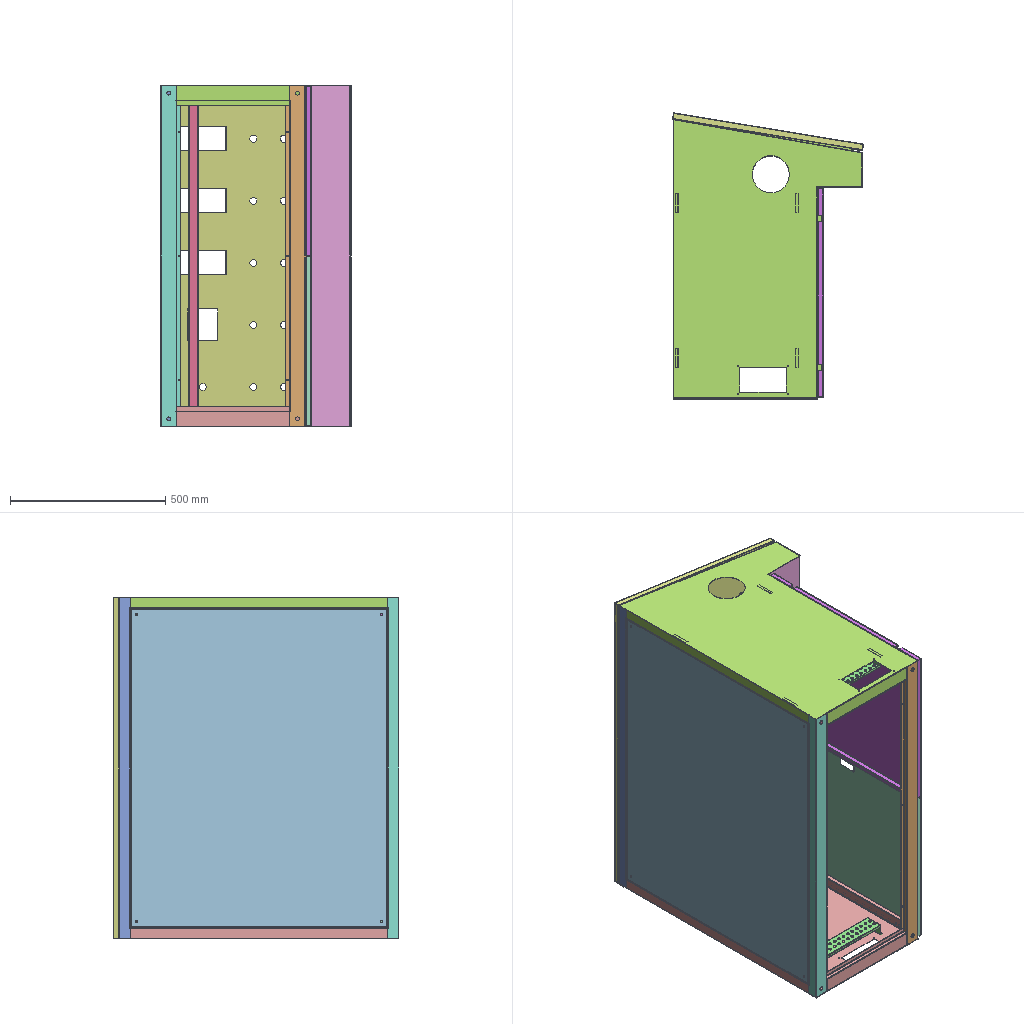Assembly | SolidWorks | 19 different items | 25 placed | box 615 x 920 x 1100 mm
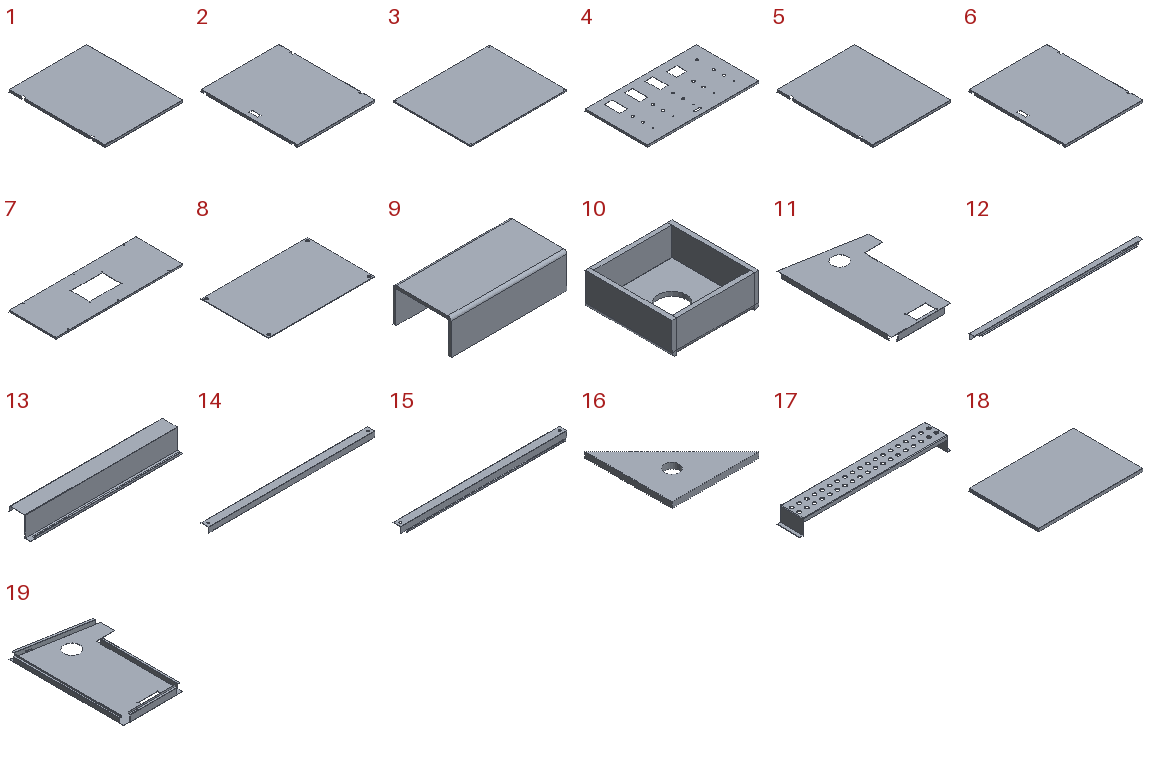Parts list (item | name | quantity | parent item | size | volume | features):
1 | (subassembly) | x1 | - | 559 x 672 x 18.5 mm | 634923 mm3 | -
2 | (subassembly) | x1 | - | 545.5 x 674 x 16.5 mm | 628405 mm3 | -
3 | - | x1 | - | 1027 x 827 x 13 mm | 1380132 mm3 | features EdgeFlange 2, FlatPattern 1, ICE 1, SMBaseFlange 1, SheetMetal 1
4 | - | x1 | - | 1100 x 620 x 20 mm | 1080338 mm3 | features EdgeFlange 2, ICE 2, FlatPattern 1, SMBaseFlange 1, SheetMetal 1
5 | - | x1 | in 1 | 559 x 672 x 18.5 mm | 634923 mm3 | features EdgeFlange 4, ICE 2, FlatPattern 1, SMBaseFlange 1, SheetMetal 1
6 | - | x1 | in 2 | 545.5 x 674 x 16.5 mm | 628405 mm3 | features ICE 3, EdgeFlange 2, FlatPattern 1, SMBaseFlange 1, SheetMetal 1
7 | - | x1 | - | 1010 x 375 x 12 mm | 553312 mm3 | features ICE 2, EdgeFlange 1, FlatPattern 1, SMBaseFlange 1, SheetMetal 1
8 | - | x1 | - | 275 x 175 x 1.5 mm | 71957 mm3 | features FlatPattern 1, ICE 1, SMBaseFlange 1, SheetMetal 1
9 | - | x1 | - | 60 x 30 x 18 mm | 5604 mm3 | features EdgeFlange 1, FlatPattern 1, SMBaseFlange 1, SheetMetal 1
10 | - | x1 | - | 40 x 40 x 15 mm | 6733 mm3 | features EdgeFlange 2, FlatPattern 1, ICE 1, SMBaseFlange 1, SheetMetal 1
11 | - | x1 | - | 610 x 910.172 x 63.5 mm | 799310 mm3 | features MirrorStock 1
12 | - | x1 | - | 1097 x 57.715 x 37.08 mm | 185139 mm3 | features EdgeFlange 5, FlatPattern 1, SMBaseFlange 1, SheetMetal 1
13 | - | x1 | - | 1097 x 172.327 x 146.5 mm | 612727 mm3 | features EdgeFlange 7, SMBaseFlange 3, FlatPattern 1, SheetMetal 1
14 | - | x1 | - | 1097 x 63.5 x 45.5 mm | 210913 mm3 | features EdgeFlange 5, ICE 2, FlatPattern 1, SMBaseFlange 1, SheetMetal 1
15 | - | x1 | - | 1097 x 78.5 x 40 mm | 218985 mm3 | features EdgeFlange 5, ICE 2, SMBaseFlange 2, FlatPattern 1, SheetMetal 1
16 | - | x4 | - | 30 x 30 x 2 mm | 859.144 mm3 | features FlatPattern 1, SMBaseFlange 1, SheetMetal 1
17 | - | x4 | - | 397 x 60 x 40 mm | 48098 mm3 | features EdgeFlange 3, FlatPattern 1, ICE 1, SMBaseFlange 1, SheetMetal 1
18 | - | x1 | - | 1016 x 680 x 30 mm | 1623193 mm3 | features EdgeFlange 2, FlatPattern 1, ICE 1, SMBaseFlange 1, SheetMetal 1
19 | - | x1 | - | 610 x 910.172 x 63.5 mm | 799310 mm3 | features EdgeFlange 12, ICE 6, FlatPattern 1, SMBaseFlange 1, SheetMetal 1
Mates (type | each side: item.copy, entity, surface, feature):
Coincident | 19.1 face plane Edge-Flange2 | 12.1 face plane Base-Flange1
Coincident | 19.1 face plane Base-Flange1 | 12.1 face plane Base-Flange1
Coincident | 19.1 face plane Edge-Flange3 | 12.1 face plane Edge-Flange1
Coincident | 12.1 face plane Edge-Flange1 | 11.1 face plane PAXX-457-001 Mirror | 2 times
Coincident | 12.1 face plane Base-Flange1 | 11.1 face plane PAXX-457-001 Mirror
Coincident | 19.1 face plane Base-Flange1 | 13.1 face plane Base-Flange1 | 2 times
Coincident | 19.1 face plane Cut-Extrude2 | 13.1 face plane Edge-Flange4
Coincident | 19.1 face plane Edge-Flange2 | 14.1 face plane Edge-Flange1
Coincident | 19.1 face plane Edge-Flange10 | 14.1 face plane Base-Flange1
Coincident | 19.1 face plane Base-Flange1 | 14.1 face plane Base-Flange1
Coincident | 11.1 face plane PAXX-457-001 Mirror | 15.1 face plane Edge-Flange1
Coincident | 11.1 face plane PAXX-457-001 Mirror | 15.1 face plane Base-Flange1 | 2 times
Coincident | 19.1 face plane Edge-Flange7 | 16.1 face plane Base-Flange1 | 2 times
Coincident | 12.1 face plane Edge-Flange5 | 16.1 face plane Base-Flange1
Coincident | 16.1 face plane Base-Flange1 | 16.2 face plane Base-Flange1
Coincident | 14.1 face plane Edge-Flange3 | 16.2 face plane Base-Flange1
Coincident | 19.1 face plane Edge-Flange7 | 16.2 face plane Base-Flange1
Coincident | 16.3 face plane Base-Flange1 | 16.4 face plane Base-Flange1
Coincident | 16.2 face plane Base-Flange1 | 16.3 face plane Base-Flange1
Coincident | 14.1 face plane Edge-Flange3 | 16.3 face plane Base-Flange1
Coincident | 11.1 face plane PAXX-457-001 Mirror | 16.3 face plane Base-Flange1
Coincident | 11.1 face plane PAXX-457-001 Mirror | 16.4 face plane Base-Flange1
Coincident | 12.1 face plane Edge-Flange5 | 16.4 face plane Base-Flange1
Coincident | 19.1 face plane Base-Flange1 | 17.1 face plane Edge-Flange2
Coincident | 19.1 face plane Edge-Flange7 | 17.1 face plane Edge-Flange1
DistanceDim | 17.1 face plane Edge-Flange3 | 15.1 face plane Base-Flange1
Coincident | 17.1 face plane Edge-Flange1 | 17.2 face plane Edge-Flange1
Coincident | 17.1 face plane Edge-Flange3 | 17.2 face plane Edge-Flange3
Coincident | 11.1 face plane PAXX-457-001 Mirror | 17.2 face plane Edge-Flange2
Coincident | 17.1 face plane Base-Flange1 | 18.1 face plane Edge-Flange1
Concentric | 17.2 face cylinder Cut-Extrude1 | 18.1 face cylinder Cut-Extrude1 | 2 times
Concentric | 16.1 face cylinder Base-Flange1 | 3.1 face cylinder Cut-Extrude1
Concentric | 16.4 face cylinder Base-Flange1 | 3.1 face cylinder Cut-Extrude1
Coincident | 11.1 face plane PAXX-457-001 Mirror | 3.1 face plane Base-Flange1
Coincident | 11.1 edge | 4.1 edge
Coincident | 11.1 face plane PAXX-457-001 Mirror | 4.1 face plane Edge-Flange1
Coincident | 5.1 face plane Base-Flange1 | 6.1 face plane Base-Flange1